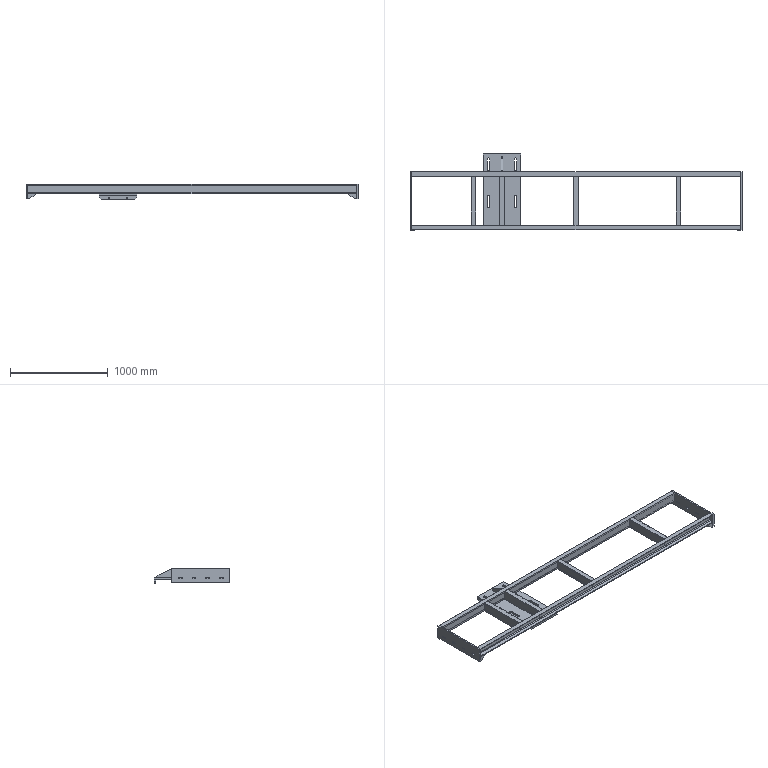Part | SolidWorks | features ICE 7, MirrorSolid 2, Chamfer 1, MoveFace 1, WeldMemberFeat 1, WeldmentFeature 1 | 15 solids | 205 faces | box 3390 x 776 x 160 mm | volume 20064178 mm3 | plane 153 | cylinder 52 | commonest cylinder face diameters 18 x16 8.4 x12 17 x12 22 x8 12 x4